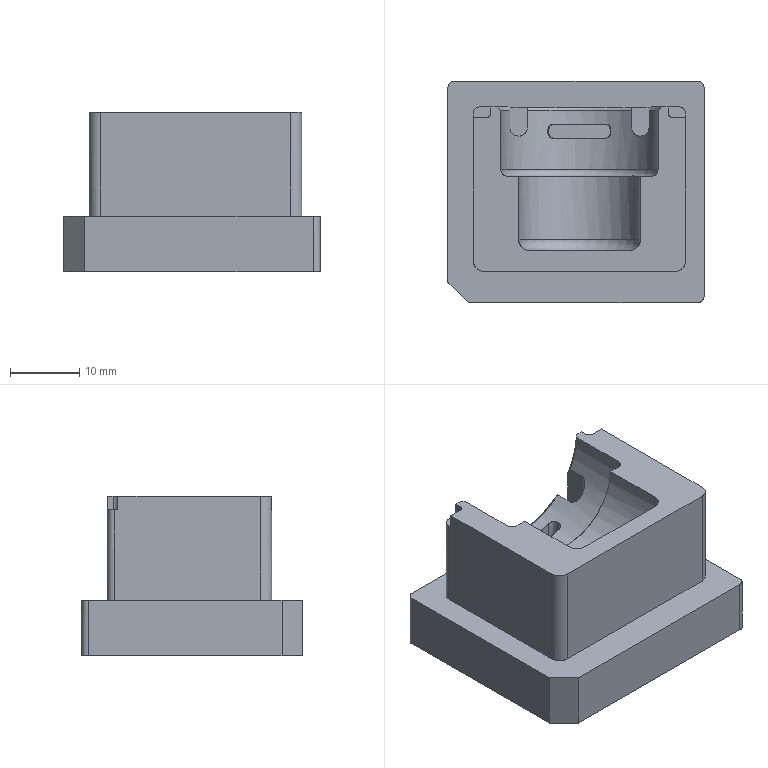NC program | PowerMill | posted with a generic post | part box 37 x 32 x 23 mm
Lines 26493 to 27420 of 253511:
N26590 M6
N26591 S8500 M03
N26592 G00 G90 X0.0 Y0.0
N26593 G43 Z11.8 H3
N26594
N26595 G05 P10000 R8
N26596 X-13.2853 Y23.0094
N26597 Z-1.026
N26598 G01 Z-2.226 F360.0
N26599 X-13.285 Y17.7344 F600.0
N26600 X-13.4122 Y17.5229
N26601 G00 Z2.8456
N26602 G01 X-25.6135 Y10.8449 F10000.0
N26603 G00 Z-1.026
N26604 G01 Z-2.226 F360.0
N26605 X-20.3385 Y10.845 F600.0
N26606 G03 X-20.22 Y11.144 I-0.4782 J0.3625
N26607 G01 X-20.1914 Y11.413
N26608 X-20.146 Y11.6959
N26609 X-20.0847 Y11.9789
N26610 X-20.0072 Y12.2619
N26611 X-19.9128 Y12.5448
N26612 X-19.806 Y12.8144
N26613 X-19.6686 Y13.1108
N26614 X-19.5161 Y13.3937
N26615 X-19.3407 Y13.6767
N26616 X-19.1212 Y13.9832
N26617 X-18.9083 Y14.2427
N26618 X-18.7427 Y14.4237
N26619 X-18.5607 Y14.6047
N26620 X-18.333 Y14.8086
N26621 X-18.1665 Y14.9439
N26622 X-18.0001 Y15.0683
N26623 X-17.7616 Y15.2304
N26624 X-17.5233 Y15.3745
N26625 X-17.1593 Y15.5642
N26626 X-16.879 Y15.6871
N26627 X-16.5988 Y15.7917
N26628 X-16.4285 Y15.8448
N26629 G03 X-16.1832 Y15.9931 I-0.1787 J0.5728
N26630 G01 X-15.9969 Y16.1791
N26631 X-15.7579 Y16.3903
N26632 X-15.6131 Y16.5064
N26633 X-15.4053 Y16.6597
N26634 X-15.1974 Y16.7985
N26635 X-14.9542 Y16.9441
N26636 X-14.6368 Y17.1088
N26637 X-14.3566 Y17.2332
N26638 X-14.0763 Y17.3387
N26639 X-13.796 Y17.4272
N26640 X-13.4678 Y17.5089
N26641 G03 X-13.1084 Y17.7344 I-0.1185 J0.5882
N26642 G00 Z2.8456
N26643 G01 X14.0761 Y23.0093 F10000.0
N26644 G00 Z-1.026
N26645 G01 Z-2.226 F360.0
N26646 X14.1038 Y17.7344 F600.0
N26647 G03 X14.4632 Y17.509 I0.4779 J0.3628
N26648 G01 X14.7919 Y17.4272
N26649 X15.0722 Y17.3387
N26650 X15.3524 Y17.2332
N26651 X15.7072 Y17.0723
N26652 X15.9501 Y16.9441
N26653 X16.1933 Y16.7985
N26654 X16.401 Y16.6602
N26655 X16.609 Y16.5064
N26656 X16.7538 Y16.3903
N26657 X16.9926 Y16.1791
N26658 X17.1791 Y15.9929
N26659 G03 X17.4244 Y15.8448 I0.4239 J0.4247
N26660 G01 X17.5946 Y15.7917
N26661 X17.8749 Y15.6871
N26662 X18.1552 Y15.5642
N26663 X18.4355 Y15.4212
N26664 X18.5192 Y15.3745
N26665 X18.7575 Y15.2304
N26666 X18.996 Y15.0683
N26667 X19.1623 Y14.9439
N26668 X19.3288 Y14.8086
N26669 X19.5566 Y14.6047
N26670 X19.7387 Y14.4235
N26671 X19.9042 Y14.2427
N26672 X20.1171 Y13.9832
N26673 X20.3366 Y13.6767
N26674 X20.512 Y13.3937
N26675 X20.6776 Y13.0843
N26676 X20.802 Y12.8144
N26677 X20.9087 Y12.5448
N26678 X21.003 Y12.2619
N26679 X21.0805 Y11.9789
N26680 X21.1417 Y11.6959
N26681 X21.1873 Y11.413
N26682 X21.216 Y11.1437
N26683 G03 X21.3344 Y10.845 I0.5966 J0.0636
N26684 G00 Z4.0
N26685 G01 X-18.9684 Y20.7053 F10000.0
N26686 G00 Z0.93
N26687 G01 Z-0.27 F360.0
N26688 X-15.7068 Y16.5595 F600.0
N26689 X-15.7124 Y-16.5405
N26690 X-15.3606 Y-16.6606
N26691 X-15.0444 Y-16.751
N26692 X-14.7189 Y-16.8277
N26693 X-14.3786 Y-16.8904
N26694 X-14.0778 Y-16.9323
N26695 X-13.7808 Y-16.9601
N26696 X-13.4371 Y-16.9771
N26697 X-13.121 Y-16.98
N26698 X-11.0818
N26699 X-11.076 Y17.7265
N26700 G02 X-10.3716 Y17.6448 I-0.3012 J-5.6728
N26701 G01 X-10.3158 Y17.6324
N26702 G02 X-9.8419 Y17.5204 I-0.9529 J-5.0895
N26703 G01 X-9.5616 Y17.4312
N26704 X-9.271 Y17.321
N26705 X-8.9172 Y17.1605
N26706 X-8.6536 Y17.0197
N26707 X-8.4152 Y16.8769
N26708 X-8.2109 Y16.7402
N26709 X-8.0028 Y16.5869
N26710 G02 X-7.6028 Y16.245 I-3.8212 J-4.8756
N26711 G01 X-7.0427 Y15.6887
N26712 X-6.8034 Y15.4407
N26713 X-6.7118 Y15.3375
N26714 X-6.4832 Y15.0548
N26715 X-6.4458 Y15.0045
N26716 X-6.4511 Y-16.98
N26717 X-1.8205
N26718 X-1.8181 Y-3.0199
N26719 X2.8126 Y-3.02
N26720 X2.8102 Y-16.98
N26721 X7.4409
N26722 X7.4463 Y15.0081
N26723 X7.5171 Y15.1047
N26724 X7.6921 Y15.3185
N26725 X7.803 Y15.4446
N26726 X7.9891 Y15.6394
N26727 X8.5988 Y16.2451
N26728 G02 X8.9953 Y16.5843 I4.2011 J-4.5099
N26729 G01 X9.2068 Y16.7402
N26730 X9.4111 Y16.8769
N26731 X9.6666 Y17.0298
N26732 X9.9866 Y17.1963
N26733 X10.2422 Y17.3101
N26734 X10.3997 Y17.3738
N26735 X10.5594 Y17.4319
N26736 X10.8431 Y17.5219
N26737 X11.1234 Y17.5942
N26738 G02 X12.0774 Y17.7269 I1.2453 J-5.4572
N26739 G01 X12.0716 Y-16.98
N26740 X14.3887 Y-16.9783
N26741 X14.7049 Y-16.9654
N26742 X15.0303 Y-16.9373
N26743 X15.3648 Y-16.892
N26744 X15.6714 Y-16.8366
N26745 X15.992 Y-16.7634
N26746 X16.2431 Y-16.694
N26747 X16.6337 Y-16.5681
N26748 X16.7023 Y-16.5425
N26749 X16.7079 Y16.5555
N26750 G00 Z11.8
N26751 G05 P0
N26752 (---------------)
N26753 ( END TOOLPATH : 精公基准台01-平坦面平行-D10 )
N26754 (---------------)
N26755 ( START TOOLPATH : 精公基准台01-基准面偏置-D10 )
N26756 (---------------)
N26757 G00 X0.0 Y0.0 Z9.8
N26758 G05 P10000 R8
N26759 X8.2525 Y26.7548
N26760 Z-14.0
N26761 G01 Z-15.2 F360.0
N26762 Y21.4798 F600.0
N26763 X0.562 Y17.6345
N26764 X14.8922
N26765 X15.4542 Y17.6062
N26766 X15.7352 Y17.5735
N26767 X16.0162 Y17.5276
N26768 X16.3987 Y17.4446
N26769 X16.5781 Y17.3974
N26770 X16.8591 Y17.3114
N26771 X17.1401 Y17.2108
N26772 X17.4211 Y17.0954
N26773 X17.7021 Y16.9632
N26774 X17.8823 Y16.8696
N26775 X18.0598 Y16.7711
N26776 X18.2641 Y16.647
N26777 X18.4984 Y16.4902
N26778 X18.7344 Y16.3192
N26779 X18.826 Y16.2477
N26780 X19.1 Y16.0145
N26781 X19.3754 Y15.7565
N26782 X19.6432 Y15.4681
N26783 X19.8731 Y15.1937
N26784 X19.95 Y15.0937
N26785 X20.1155 Y14.8615
N26786 X20.2677 Y14.631
N26787 X20.3967 Y14.4152
N26788 X20.5803 Y14.0683
N26789 X20.7105 Y13.7869
N26790 X20.8237 Y13.5055
N26791 X20.9228 Y13.2242
N26792 X21.0072 Y12.9428
N26793 X21.0739 Y12.6763
N26794 X21.1337 Y12.3801
N26795 X21.196 Y11.956
N26796 X21.2152 Y11.7463
N26797 X21.2273 Y11.536
N26798 X21.2347 Y11.2546
N26799 Y-9.5664
N26800 X21.2298 Y-10.1291
N26801 X21.2161 Y-10.4105
N26802 X21.1894 Y-10.6919
N26803 X21.1515 Y-10.9732
N26804 X21.1016 Y-11.2546
N26805 X21.0739 Y-11.3884
N26806 X20.965 Y-11.8173
N26807 X20.8791 Y-12.0987
N26808 X20.7781 Y-12.3801
N26809 X20.6653 Y-12.6614
N26810 X20.5355 Y-12.9428
N26811 X20.3799 Y-13.2467
N26812 X20.2307 Y-13.5055
N26813 X20.0959 Y-13.7203
N26814 X19.95 Y-13.935
N26815 X19.8531 Y-14.0683
N26816 X19.6333 Y-14.3488
N26817 X19.388 Y-14.6293
N26818 X19.1062 Y-14.9177
N26819 X18.8035 Y-15.1937
N26820 X18.5338 Y-15.4131
N26821 X18.2641 Y-15.6136
N26822 X18.0508 Y-15.7565
N26823 X17.7021 Y-15.9691
N26824 X17.4211 Y-16.1188
N26825 X17.1401 Y-16.2557
N26826 X16.9952 Y-16.3192
N26827 X16.5781 Y-16.4818
N26828 X16.2972 Y-16.5743
N26829 X16.0162 Y-16.6541
N26830 X15.7352 Y-16.7213
N26831 X15.4542 Y-16.7761
N26832 X15.1732 Y-16.8187
N26833 X14.8922 Y-16.8509
N26834 X14.3303 Y-16.8797
N26835 X-13.2063 Y-16.8803
N26836 X-13.7683 Y-16.8616
N26837 X-14.0493 Y-16.835
N26838 X-14.3303 Y-16.7973
N26839 X-14.6112 Y-16.7475
N26840 X-14.8922 Y-16.6863
N26841 X-15.1732 Y-16.6114
N26842 X-15.4542 Y-16.5258
N26843 X-15.7268 Y-16.4283
N26844 X-15.9994 Y-16.3192
N26845 X-16.2972 Y-16.183
N26846 X-16.5781 Y-16.04
N26847 X-16.8166 Y-15.905
N26848 X-17.1401 Y-15.7012
N26849 X-17.4211 Y-15.5033
N26850 X-17.7021 Y-15.283
N26851 X-17.8077 Y-15.1937
N26852 X-18.0359 Y-14.9887
N26853 X-18.2641 Y-14.7645
N26854 X-18.3906 Y-14.631
N26855 X-18.6193 Y-14.3702
N26856 X-18.8573 Y-14.0683
N26857 X-19.0562 Y-13.7869
N26858 X-19.2349 Y-13.5055
N26859 X-19.388 Y-13.239
N26860 X-19.5395 Y-12.9428
N26861 X-19.6691 Y-12.6614
N26862 X-19.7823 Y-12.3801
N26863 X-19.872 Y-12.1321
N26864 X-19.9692 Y-11.8173
N26865 X-20.0442 Y-11.536
N26866 X-20.1058 Y-11.2546
N26867 X-20.1557 Y-10.9732
N26868 X-20.1936 Y-10.6919
N26869 X-20.2199 Y-10.4105
N26870 X-20.234 Y-10.1291
N26871 X-20.2386 Y-9.5664
N26872 Y11.2546
N26873 X-20.2312 Y11.536
N26874 X-20.2137 Y11.8173
N26875 X-20.1827 Y12.0987
N26876 X-20.1379 Y12.3801
N26877 X-20.0815 Y12.6614
N26878 X-20.0112 Y12.9428
N26879 G02 X-19.8279 Y13.5055 I6.0813 J-1.6696
N26880 G01 X-19.7146 Y13.7869
N26881 X-19.5845 Y14.0683
N26882 X-19.388 Y14.4373
N26883 X-19.2719 Y14.631
N26884 X-19.0846 Y14.9124
N26885 X-18.8773 Y15.1937
N26886 X-18.6129 Y15.5066
N26887 X-18.3793 Y15.7565
N26888 X-18.2641 Y15.8688
N26889 X-18.0005 Y16.1061
N26890 X-17.7021 Y16.3469
N26891 X-17.4211 Y16.5459
N26892 X-17.1401 Y16.7258
N26893 X-16.8635 Y16.8819
N26894 X-16.5781 Y17.0259
N26895 X-16.2972 Y17.1502
N26896 X-16.0162 Y17.2584
N26897 X-15.7352 Y17.3523
N26898 X-15.4029 Y17.4446
N26899 X-15.1476 Y17.5031
N26900 X-14.8922 Y17.5496
N26901 X-14.6112 Y17.5901
N26902 X-14.3303 Y17.6167
N26903 X-14.0493 Y17.6313
N26904 X-13.7683 Y17.6345
N26905 X0.562
N26906 G00 Z9.8
N26907 G05 P0
N26908 (---------------)
N26909 ( END TOOLPATH : 精公基准台01-基准面偏置-D10 )
N26910 (---------------)
N26911 ( START TOOLPATH : 精公基准台01-外形侧光-D10 )
N26912 (---------------)
N26913 G00 X0.0 Y0.0 Z10.8
N26914 G05 P10000 R8
N26915 X19.7601 Y-14.4265
N26916 Z-13.97
N26917 G01 Z-15.17 F360.0
N26918 G03 X18.678 Y-14.8101 I-0.078 J-1.498 F600.0
N26919 G02 X14.2394 Y-16.51 I-4.4264 J4.913
N26920 G01 X-13.3291 Y-16.5095
N26921 G02 X-19.8686 Y-9.858 I0.073 J6.6122
N26922 G01 X-19.8681 Y11.321
N26923 G02 X-13.8743 Y17.2645 I6.0119 J-0.0688
N26924 G01 X0.4564
N26925 X14.7877
N26926 G02 X20.864 Y11.3185 I0.0632 J-6.0131
N26927 G01 X20.8644 Y-9.8589
N26928 G02 X18.678 Y-14.8101 I-6.6128 J-0.0382
N26929 G03 X18.1841 Y-15.8464 I1.0041 J-1.1144
N26930 G01 X19.6988 Y-14.3765
N26931 G03 X18.6161 Y-14.7582 I-0.0806 J-1.4979
N26932 G02 X14.2395 Y-16.43 I-4.3645 J4.8611
N26933 G01 X14.2394
N26934 X-13.3266 Y-16.4295
N26935 G02 X-19.7886 Y-9.858 I0.0705 J6.5322
N26936 G01 X-19.7881 Y11.3185
N26937 G02 X-13.8743 Y17.1845 I5.9318 J-0.0663
N26938 G01 X0.4564
N26939 X14.7871
N26940 G02 X20.784 Y11.3185 I0.0639 J-5.9331
N26941 G01 X20.7844 Y-9.858
N26942 G02 X18.6161 Y-14.7582 I-6.5328 J-0.0391
N26943 G03 X18.1204 Y-15.7937 I1.0021 J-1.1162
N26944 G00 Z10.8
N26945 G05 P0
N26946 (---------------)
N26947 ( END TOOLPATH : 精公基准台01-外形侧光-D10 )
N26948 (---------------)
N26949 ( START TOOLPATH : 精公基准台01-基准台侧光-D10 )
N26950 (---------------)
N26951 G00 X0.0 Y0.0 Z9.8
N26952 G05 P10000 R8
N26953 X23.9441 Y-24.0122
N26954 Z-21.9
N26955 G01 Z-23.1 F360.0
N26956 G03 X20.9858 Y-19.9813 I-1.4792 J2.0155 F600.0
N26957 G01 X20.9853 Y-19.9816
N26958 X20.9833 Y-19.9831
N26959 X20.9812 Y-19.9844
N26960 X20.5928 Y-20.2345
N26961 X20.5911 Y-20.2356
N26962 X20.5893 Y-20.2366
N26963 X20.4744 Y-20.3027
N26964 X20.4733 Y-20.3033
N26965 X20.4723 Y-20.3038
N26966 X20.2711 Y-20.4116
N26967 X20.2694 Y-20.4125
N26968 X20.2677 Y-20.4133
N26969 X19.9516 Y-20.5638
N26970 X19.9494 Y-20.5648
N26971 X19.9473 Y-20.5657
N26972 X19.6312 Y-20.6942
N26973 X19.6291 Y-20.695
N26974 X19.6269 Y-20.6958
N26975 X19.3108 Y-20.804
N26976 X19.3087 Y-20.8047
N26977 X19.3066 Y-20.8053
N26978 X18.9904 Y-20.8943
N26979 X18.9887 Y-20.8948
N26980 X18.987 Y-20.8952
N26981 X18.781 Y-20.9435
N26982 X18.7799 Y-20.9438
N26983 X18.7788 Y-20.944
N26984 X18.6686 Y-20.9665
N26985 X18.6672 Y-20.9667
N26986 X18.6659 Y-20.967
N26987 X18.3497 Y-21.0203
N26988 X18.3476 Y-21.0206
N26989 X18.3455 Y-21.0209
N26990 X18.0293 Y-21.0567
N26991 X18.0272 Y-21.057
N26992 X18.025 Y-21.0571
N26993 X17.7089 Y-21.0757
N26994 X17.707 Y-21.0758
N26995 X17.7052
N26996 X17.3891 Y-21.08
N26997 X17.3885
N26998 X17.388
N26999 X-15.4911
N27000 X-15.4923
N27001 X-15.4935
N27002 X-15.8097 Y-21.0705
N27003 X-15.8122 Y-21.0704
N27004 X-15.8147 Y-21.0702
N27005 X-16.1309 Y-21.0406
N27006 X-16.1334 Y-21.0404
N27007 X-16.1359 Y-21.04
N27008 X-16.4521 Y-20.9899
N27009 X-16.4546 Y-20.9895
N27010 X-16.4571 Y-20.989
N27011 X-16.7733 Y-20.9178
N27012 X-16.7758 Y-20.9172
N27013 X-16.7783 Y-20.9165
N27014 X-17.0945 Y-20.8232
N27015 X-17.097 Y-20.8224
N27016 X-17.0996 Y-20.8216
N27017 X-17.4157 Y-20.7049
N27018 X-17.4177 Y-20.7041
N27019 X-17.4197 Y-20.7033
N27020 X-17.6059 Y-20.6229
N27021 X-17.6072 Y-20.6224
N27022 X-17.6084 Y-20.6218
N27023 X-17.7384 Y-20.5603
N27024 X-17.7402 Y-20.5594
N27025 X-17.742 Y-20.5584
N27026 X-18.0581 Y-20.3888
N27027 X-18.06 Y-20.3878
N27028 X-18.0618 Y-20.3868
N27029 X-18.2021 Y-20.3017
N27030 X-18.2034 Y-20.301
N27031 X-18.2046 Y-20.3001
N27032 X-18.3804 Y-20.1844
N27033 X-18.3822 Y-20.1832
N27034 X-18.384 Y-20.1819
N27035 X-18.655 Y-19.9815
N27036 X-18.6575 Y-19.9795
N27037 X-18.66 Y-19.9774
N27038 X-19.0215 Y-19.6612
N27039 X-19.0234 Y-19.6595
N27040 X-19.0254 Y-19.6576
N27041 X-21.8719 Y-16.8123
N27042 X-21.872 Y-16.8122
N27043 X-21.8721 Y-16.8121
N27044 X-22.1858 Y-16.4959
N27045 X-22.1876 Y-16.494
N27046 X-22.1893 Y-16.4921
N27047 X-22.4647 Y-16.176
N27048 X-22.4668 Y-16.1735
N27049 X-22.4688 Y-16.1709
N27050 X-22.7019 Y-15.8548
N27051 X-22.7034 Y-15.8527
N27052 X-22.7048 Y-15.8507
N27053 X-22.8297 Y-15.657
N27054 X-22.8305 Y-15.6558
N27055 X-22.8313 Y-15.6545
N27056 X-22.904 Y-15.532
N27057 X-22.905 Y-15.5302
N27058 X-22.906 Y-15.5285
N27059 X-23.0729 Y-15.2123
N27060 X-23.0739 Y-15.2104
N27061 X-23.0748 Y-15.2085
N27062 X-23.1513 Y-15.0425
N27063 X-23.1519 Y-15.0412
N27064 X-23.1524 Y-15.04
N27065 X-23.2154 Y-14.8898
N27066 X-23.2162 Y-14.8879
N27067 X-23.2169 Y-14.8861
N27068 X-23.3313 Y-14.5699
N27069 X-23.3322 Y-14.5674
N27070 X-23.3329 Y-14.5649
N27071 X-23.4241 Y-14.2487
N27072 X-23.4248 Y-14.2462
N27073 X-23.4254 Y-14.2437
N27074 X-23.4946 Y-13.9275
N27075 X-23.4951 Y-13.925
N27076 X-23.4955 Y-13.9225
N27077 X-23.5437 Y-13.6063
N27078 X-23.544 Y-13.6038
N27079 X-23.5443 Y-13.6012
N27080 X-23.572 Y-13.2851
N27081 X-23.5721 Y-13.2826
N27082 X-23.5722 Y-13.2801
N27083 X-23.58 Y-12.9639
N27084 Y-12.963
N27085 Y-12.962
N27086 Y14.8588
N27087 Y14.8592
N27088 Y14.8596
N27089 X-23.577 Y15.1758
N27090 X-23.5769 Y15.1775
N27091 X-23.5768 Y15.1793
N27092 X-23.5597 Y15.4955
N27093 X-23.5596 Y15.4976
N27094 X-23.5594 Y15.4998
N27095 X-23.525 Y15.8159
N27096 X-23.5247 Y15.818
N27097 X-23.5244 Y15.8201
N27098 X-23.4737 Y16.1314
N27099 X-23.4734 Y16.1335
N27100 X-23.4729 Y16.1356
N27101 X-23.4029 Y16.4566
N27102 X-23.4024 Y16.4588
N27103 X-23.4018 Y16.4609
N27104 X-23.3145 Y16.777
N27105 X-23.3138 Y16.7792
N27106 X-23.3131 Y16.7814
N27107 X-23.2061 Y17.0975
N27108 X-23.2056 Y17.0989
N27109 X-23.2051 Y17.1002
N27110 X-23.1535 Y17.2367
N27111 X-23.153 Y17.2379
N27112 X-23.1525 Y17.239
N27113 X-23.0782 Y17.4186
N27114 X-23.0774 Y17.4204
N27115 X-23.0766 Y17.4221
N27116 X-22.9277 Y17.7382
N27117 X-22.927 Y17.7398
N27118 X-22.9262 Y17.7413
N27119 X-22.8334 Y17.9185
N27120 X-22.8328 Y17.9196
N27121 X-22.8322 Y17.9206
N27122 X-22.7541 Y18.0595
N27123 X-22.7532 Y18.0611
N27124 X-22.7522 Y18.0627
N27125 X-22.5547 Y18.3788
N27126 X-22.5533 Y18.381
N27127 X-22.5518 Y18.3831
N27128 X-22.3251 Y18.6992
N27129 X-22.3239 Y18.7008
N27130 X-22.3227 Y18.7024
N27131 X-22.1928 Y18.8657
N27132 X-22.1919 Y18.8667
N27133 X-22.1911 Y18.8678
N27134 X-22.0608 Y19.0206
N27135 X-22.0597 Y19.0218
N27136 X-22.0587 Y19.023
N27137 X-21.8728 Y19.2242
N27138 X-21.8718 Y19.2253
N27139 X-21.8708 Y19.2263
N27140 X-21.7567 Y19.3413
N27141 X-21.7556 Y19.3423
N27142 X-21.7546 Y19.3433
N27143 X-21.5526 Y19.5324
N27144 X-21.5513 Y19.5335
N27145 X-21.5501 Y19.5347
N27146 X-21.4024 Y19.6617
N27147 X-21.4015 Y19.6624
N27148 X-21.4006 Y19.6632
N27149 X-21.2321 Y19.7997
N27150 X-21.2307 Y19.8009
N27151 X-21.2292 Y19.802
N27152 X-20.9853 Y19.9816
N27153 X-20.9833 Y19.9831
N27154 X-20.9812 Y19.9844
N27155 X-20.5928 Y20.2345
N27156 X-20.5911 Y20.2356
N27157 X-20.5893 Y20.2366
N27158 X-20.4744 Y20.3027
N27159 X-20.4733 Y20.3033
N27160 X-20.4723 Y20.3038
N27161 X-20.2711 Y20.4116
N27162 X-20.2694 Y20.4125
N27163 X-20.2677 Y20.4133
N27164 X-19.9516 Y20.5638
N27165 X-19.9494 Y20.5648
N27166 X-19.9473 Y20.5657
N27167 X-19.6312 Y20.6942
N27168 X-19.6291 Y20.695
N27169 X-19.6269 Y20.6958
N27170 X-19.3108 Y20.804
N27171 X-19.3087 Y20.8047
N27172 X-19.3066 Y20.8053
N27173 X-18.9904 Y20.8943
N27174 X-18.9883 Y20.8949
N27175 X-18.9862 Y20.8954
N27176 X-18.6701 Y20.9662
N27177 X-18.668 Y20.9666
N27178 X-18.6659 Y20.967
N27179 X-18.3497 Y21.0203
N27180 X-18.3476 Y21.0206
N27181 X-18.3455 Y21.0209
N27182 X-18.0293 Y21.0567
N27183 X-18.0272 Y21.057
N27184 X-18.025 Y21.0571
N27185 X-17.7089 Y21.0757
N27186 X-17.707 Y21.0758
N27187 X-17.7052
N27188 X-17.3891 Y21.08
N27189 X-17.3885
N27190 X-17.388
N27191 X0.0
N27192 X17.388
N27193 X17.3885
N27194 X17.389
N27195 X17.7052 Y21.076
N27196 X17.707
N27197 X17.7089 Y21.0759
N27198 X18.025 Y21.0573
N27199 X18.0272 Y21.0571
N27200 X18.0294 Y21.0569
N27201 X18.3455 Y21.0208
N27202 X18.3476 Y21.0206
N27203 X18.3497 Y21.0203
N27204 X18.6658 Y20.9672
N27205 X18.668 Y20.9668
N27206 X18.6701 Y20.9663
N27207 X18.9862 Y20.8954
N27208 X18.9883 Y20.8949
N27209 X18.9904 Y20.8944
N27210 X19.3066 Y20.8053
N27211 X19.3088 Y20.8047
N27212 X19.311 Y20.804
N27213 X19.6271 Y20.695
N27214 X19.6285 Y20.6945
N27215 X19.63 Y20.6939
N27216 X19.81 Y20.624
N27217 X19.8112 Y20.6236
N27218 X19.8124 Y20.6231
N27219 X19.9485 Y20.5652
N27220 X19.9501 Y20.5645
N27221 X19.9517 Y20.5637
N27222 X20.2679 Y20.4124
N27223 X20.2694 Y20.4116
N27224 X20.2709 Y20.4109
N27225 X20.472 Y20.304
N27226 X20.4732 Y20.3033
N27227 X20.4744 Y20.3027
N27228 X20.5893 Y20.2366
N27229 X20.5908 Y20.2357
N27230 X20.5923 Y20.2348
N27231 X20.9084 Y20.0347
N27232 X20.9105 Y20.0333
N27233 X20.9126 Y20.0319
N27234 X21.2288 Y19.8023
N27235 X21.2304 Y19.8011
N27236 X21.232 Y19.7998
N27237 X21.4013 Y19.6633
N27238 X21.4023 Y19.6624
N27239 X21.4034 Y19.6615
N27240 X21.5502 Y19.5345
N27241 X21.5514 Y19.5335
N27242 X21.5526 Y19.5324
N27243 X21.7546 Y19.3433
N27244 X21.7556 Y19.3423
N27245 X21.7567 Y19.3412
N27246 X21.8708 Y19.2262
N27247 X21.8718 Y19.2251
N27248 X21.8728 Y19.2241
N27249 X22.0586 Y19.023
N27250 X22.0597 Y19.0218
N27251 X22.0608 Y19.0206
N27252 X22.1911 Y18.8673
N27253 X22.1919 Y18.8663
N27254 X22.1927 Y18.8654
N27255 X22.3227 Y18.7025
N27256 X22.3238 Y18.701
N27257 X22.3249 Y18.6995
N27258 X22.5111 Y18.4423
N27259 X22.5125 Y18.4403
N27260 X22.5139 Y18.4382
N27261 X22.7519 Y18.0632
N27262 X22.7533 Y18.0608
N27263 X22.7547 Y18.0585
N27264 X22.9263 Y17.7423
N27265 X22.9274 Y17.7402
N27266 X22.9285 Y17.7381
N27267 X23.0767 Y17.422
N27268 X23.0776 Y17.4199
N27269 X23.0785 Y17.4178
N27270 X23.2052 Y17.1016
N27271 X23.206 Y17.0995
N27272 X23.2068 Y17.0974
N27273 X23.3132 Y16.7812
N27274 X23.3138 Y16.7791
N27275 X23.3144 Y16.777
N27276 X23.4018 Y16.4609
N27277 X23.4023 Y16.4588
N27278 X23.4028 Y16.4566
N27279 X23.4718 Y16.1405
N27280 X23.4722 Y16.1384
N27281 X23.4726 Y16.1364
N27282 X23.5244 Y15.8202
N27283 X23.5247 Y15.8181
N27284 X23.525 Y15.8159
N27285 X23.5591 Y15.4997
N27286 X23.5593 Y15.4976
N27287 X23.5595 Y15.4955
N27288 X23.5768 Y15.1794
N27289 X23.5769 Y15.1776
N27290 Y15.1758
N27291 X23.58 Y14.8596
N27292 Y14.8592
N27293 Y14.8588
N27294 Y-14.8588
N27295 Y-14.8592
N27296 Y-14.8596
N27297 X23.577 Y-15.1758
N27298 X23.5769 Y-15.1775
N27299 X23.5768 Y-15.1793
N27300 X23.5597 Y-15.4955
N27301 X23.5596 Y-15.4976
N27302 X23.5594 Y-15.4998
N27303 X23.525 Y-15.8159
N27304 X23.5247 Y-15.818
N27305 X23.5244 Y-15.8201
N27306 X23.4737 Y-16.1314
N27307 X23.4734 Y-16.1335
N27308 X23.4729 Y-16.1356
N27309 X23.4029 Y-16.4566
N27310 X23.4024 Y-16.4588
N27311 X23.4018 Y-16.4609
N27312 X23.3145 Y-16.777
N27313 X23.3138 Y-16.7792
N27314 X23.3131 Y-16.7814
N27315 X23.2061 Y-17.0975
N27316 X23.2056 Y-17.0989
N27317 X23.2051 Y-17.1002
N27318 X23.1535 Y-17.2367
N27319 X23.153 Y-17.2379
N27320 X23.1525 Y-17.239
N27321 X23.0782 Y-17.4186
N27322 X23.0774 Y-17.4204
N27323 X23.0766 Y-17.4221
N27324 X22.9277 Y-17.7382
N27325 X22.927 Y-17.7398
N27326 X22.9262 Y-17.7413
N27327 X22.8334 Y-17.9185
N27328 X22.8328 Y-17.9196
N27329 X22.8322 Y-17.9206
N27330 X22.7541 Y-18.0595
N27331 X22.7532 Y-18.0611
N27332 X22.7522 Y-18.0627
N27333 X22.5547 Y-18.3788
N27334 X22.5533 Y-18.381
N27335 X22.5518 Y-18.3831
N27336 X22.3251 Y-18.6992
N27337 X22.3239 Y-18.7008
N27338 X22.3227 Y-18.7024
N27339 X22.1928 Y-18.8657
N27340 X22.1919 Y-18.8667
N27341 X22.1911 Y-18.8678
N27342 X22.0608 Y-19.0206
N27343 X22.0597 Y-19.0218
N27344 X22.0587 Y-19.023
N27345 X21.8728 Y-19.2242
N27346 X21.8718 Y-19.2253
N27347 X21.8708 Y-19.2263
N27348 X21.7567 Y-19.3413
N27349 X21.7556 Y-19.3423
N27350 X21.7546 Y-19.3433
N27351 X21.5526 Y-19.5324
N27352 X21.5513 Y-19.5335
N27353 X21.5501 Y-19.5347
N27354 X21.4024 Y-19.6617
N27355 X21.4015 Y-19.6624
N27356 X21.4006 Y-19.6632
N27357 X21.2321 Y-19.7997
N27358 X21.2307 Y-19.8009
N27359 X21.2292 Y-19.802
N27360 X20.9858 Y-19.9813
N27361 G03 X23.9508 Y-24.0072 I1.4825 J-2.0129
N27362 G01 X23.6406 Y-24.1237
N27363 G03 X20.9341 Y-19.9196 I-1.3532 J2.102
N27364 G01 X20.5495 Y-20.1672
N27365 X20.4345 Y-20.2333
N27366 X20.2333 Y-20.3411
N27367 X19.9172 Y-20.4916
N27368 X19.601 Y-20.6201
N27369 X19.2849 Y-20.7283
N27370 X18.9687 Y-20.8173
N27371 X18.7628 Y-20.8656
N27372 X18.6526 Y-20.8881
N27373 X18.3364 Y-20.9414
N27374 X18.0203 Y-20.9773
N27375 X17.7042 Y-20.9958
N27376 X17.388 Y-21.0
N27377 X-15.4911
N27378 X-15.8073 Y-20.9906
N27379 X-16.1234 Y-20.961
N27380 X-16.4396 Y-20.9109
N27381 X-16.7557 Y-20.8397
N27382 X-17.0719 Y-20.7465
N27383 X-17.388 Y-20.6299
N27384 X-17.5742 Y-20.5495
N27385 X-17.7042 Y-20.488
N27386 X-18.0203 Y-20.3183
N27387 X-18.1606 Y-20.2333
N27388 X-18.3364 Y-20.1176
N27389 X-18.6074 Y-19.9172
N27390 X-18.9688 Y-19.601
N27391 X-19.2862 Y-19.2849
N27392 X-21.8153 Y-16.7557
N27393 X-22.129 Y-16.4396
N27394 X-22.4044 Y-16.1234
N27395 X-22.6375 Y-15.8073
N27396 X-22.7625 Y-15.6137
N27397 X-22.8352 Y-15.4911
N27398 X-23.0022 Y-15.175
N27399 X-23.0786 Y-15.009
N27400 X-23.1416 Y-14.8588
N27401 X-23.2561 Y-14.5427
N27402 X-23.3472 Y-14.2266
N27403 X-23.4164 Y-13.9104
N27404 X-23.4646 Y-13.5943
N27405 X-23.4923 Y-13.2781
N27406 X-23.5 Y-12.962
N27407 Y14.8588
N27408 X-23.497 Y15.175
N27409 X-23.4799 Y15.4911
N27410 X-23.4454 Y15.8073
N27411 X-23.3948 Y16.1185
N27412 X-23.3247 Y16.4396
N27413 X-23.2374 Y16.7557
N27414 X-23.1303 Y17.0719
N27415 X-23.0786 Y17.2084
N27416 X-23.0043 Y17.388
N27417 X-22.8553 Y17.7042
N27418 X-22.7625 Y17.8814
N27419 X-22.6844 Y18.0203
N27420 X-22.4868 Y18.3364
N27421 X-22.2601 Y18.6526
N27422 X-22.1302 Y18.8159
N27423 X-21.9999 Y18.9687
N27424 X-21.8141 Y19.1699
N27425 X-21.6999 Y19.2849
N27426 X-21.4979 Y19.474
N27427 X-21.3502 Y19.601
N27428 X-21.1818 Y19.7376
N27429 X-20.9379 Y19.9172
N27430 X-20.5495 Y20.1672
N27431 X-20.4345 Y20.2333
N27432 X-20.2333 Y20.3411
N27433 X-19.9172 Y20.4916
N27434 X-19.601 Y20.6201
N27435 X-19.2849 Y20.7283
N27436 X-18.9687 Y20.8173
N27437 X-18.6526 Y20.8881
N27438 X-18.3364 Y20.9414
N27439 X-18.0203 Y20.9773
N27440 X-17.7042 Y20.9958
N27441 X-17.388 Y21.0
N27442 X0.0
N27443 X17.388
N27444 X17.7042 Y20.996
N27445 X18.0203 Y20.9774
N27446 X18.3364 Y20.9414
N27447 X18.6526 Y20.8883
N27448 X18.9687 Y20.8174
N27449 X19.2849 Y20.7283
N27450 X19.601 Y20.6194
N27451 X19.7811 Y20.5495
N27452 X19.9172 Y20.4916
N27453 X20.2333 Y20.3402
N27454 X20.4345 Y20.2333
N27455 X20.5495 Y20.1672
N27456 X20.8656 Y19.9671
N27457 X21.1818 Y19.7376
N27458 X21.3511 Y19.601
N27459 X21.4979 Y19.474
N27460 X21.6999 Y19.2849
N27461 X21.8141 Y19.1698
N27462 X21.9998 Y18.9687
N27463 X22.1302 Y18.8155
N27464 X22.2601 Y18.6526
N27465 X22.4463 Y18.3954
N27466 X22.6844 Y18.0203
N27467 X22.856 Y17.7042
N27468 X23.0043 Y17.388
N27469 X23.1309 Y17.0719
N27470 X23.2373 Y16.7557
N27471 X23.3247 Y16.4396
N27472 X23.3936 Y16.1234
N27473 X23.4454 Y15.8073
N27474 X23.4796 Y15.4911
N27475 X23.4969 Y15.175
N27476 X23.5 Y14.8588
N27477 Y-14.8588
N27478 X23.497 Y-15.175
N27479 X23.4799 Y-15.4911
N27480 X23.4454 Y-15.8073
N27481 X23.3948 Y-16.1185
N27482 X23.3247 Y-16.4396
N27483 X23.2374 Y-16.7557
N27484 X23.1303 Y-17.0719
N27485 X23.0786 Y-17.2084
N27486 X23.0043 Y-17.388
N27487 X22.8553 Y-17.7042
N27488 X22.7625 Y-17.8814
N27489 X22.6844 Y-18.0203
N27490 X22.4868 Y-18.3364
N27491 X22.2601 Y-18.6526
N27492 X22.1302 Y-18.8159
N27493 X21.9999 Y-18.9687
N27494 X21.8141 Y-19.1699
N27495 X21.6999 Y-19.2849
N27496 X21.4979 Y-19.474
N27497 X21.3502 Y-19.601
N27498 X21.1818 Y-19.7376
N27499 X20.9379 Y-19.9172
N27500 X20.9341 Y-19.9196
N27501 G03 X23.6403 Y-24.1239 I1.3531 J-2.1022
N27502 G00 Z9.8
N27503 G05 P0
N27504 (---------------)
N27505 ( END TOOLPATH : 精公基准台01-基准台侧光-D10 )
N27506 (---------------)
N27507
N27508 M05
N27509 G53 Z0.0
N27510 (---------------)
N27511 ( START TOOLPATH : 精公精光01-最佳等高-R1.5 )
N27512 (---------------)
N27513 ( TOOL NO.    :22 )
N27514 ( TOOL TYPE   : BALLNOSED)
N27515 ( TOOL ID     : R1.5_1_1)
N27516 ( TOOL DIA    : 3.0 LENGTH 67.4)
N27517 T22